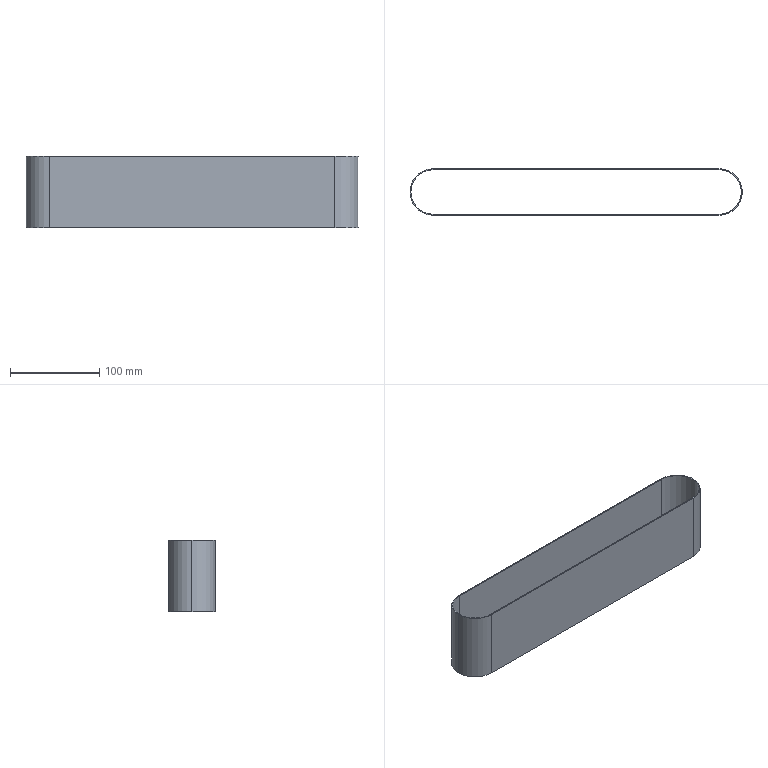Part | SolidWorks | features Extrusion 1 | 1 solid | 12 faces | box 372 x 52 x 80 mm | volume 64018 mm3 | cylinder 6 | plane 6 | commonest cylinder face diameters 50 x3 52 x3
STEP:
#1=CARTESIAN_POINT('',(0.,25.,80.));
#2=VERTEX_POINT('',#1);
#3=CARTESIAN_POINT('',(-25.,0.,80.));
#4=VERTEX_POINT('',#3);
#5=CARTESIAN_POINT('',(0.,0.,80.));
#6=DIRECTION('',(0.,0.,1.));
#7=DIRECTION('',(1.,0.,0.));
#8=AXIS2_PLACEMENT_3D('',#5,#6,#7);
#9=CIRCLE('',#8,25.);
#10=EDGE_CURVE('',#2,#4,#9,.T.);
#11=ORIENTED_EDGE('',*,*,#10,.T.);
#12=CARTESIAN_POINT('',(-25.,0.,0.));
#13=VERTEX_POINT('',#12);
#14=CARTESIAN_POINT('',(-25.,0.,80.));
#15=DIRECTION('',(0.,0.,-1.));
#16=VECTOR('',#15,1000.);
#17=LINE('',#14,#16);
#18=EDGE_CURVE('',#4,#13,#17,.T.);
#19=ORIENTED_EDGE('',*,*,#18,.T.);
#20=CARTESIAN_POINT('',(0.,25.,0.));
#21=VERTEX_POINT('',#20);
#22=CARTESIAN_POINT('',(0.,0.,0.));
#23=DIRECTION('',(0.,0.,1.));
#24=DIRECTION('',(1.,0.,0.));
#25=AXIS2_PLACEMENT_3D('',#22,#23,#24);
#26=CIRCLE('',#25,25.);
#27=EDGE_CURVE('',#21,#13,#26,.T.);
#28=ORIENTED_EDGE('',*,*,#27,.F.);
#29=CARTESIAN_POINT('',(0.,25.,80.));
#30=DIRECTION('',(0.,0.,-1.));
#31=VECTOR('',#30,1000.);
#32=LINE('',#29,#31);
#33=EDGE_CURVE('',#2,#21,#32,.T.);
#34=ORIENTED_EDGE('',*,*,#33,.F.);
#35=EDGE_LOOP('',(#11,#19,#28,#34));
#36=FACE_OUTER_BOUND('',#35,.T.);
#37=CARTESIAN_POINT('',(0.,0.,80.));
#38=DIRECTION('',(0.,0.,-1.));
#39=DIRECTION('',(-1.,0.,0.));
#40=AXIS2_PLACEMENT_3D('',#37,#38,#39);
#41=CYLINDRICAL_SURFACE('',#40,25.);
#42=ADVANCED_FACE('',(#36),#41,.F.);
#43=CARTESIAN_POINT('',(-26.,0.,80.));
#44=VERTEX_POINT('',#43);
#45=CARTESIAN_POINT('',(0.,-26.,80.));
#46=VERTEX_POINT('',#45);
#47=CARTESIAN_POINT('',(0.,0.,80.));
#48=DIRECTION('',(0.,0.,1.));
#49=DIRECTION('',(1.,0.,0.));
#50=AXIS2_PLACEMENT_3D('',#47,#48,#49);
#51=CIRCLE('',#50,26.);
#52=EDGE_CURVE('',#44,#46,#51,.T.);
#53=ORIENTED_EDGE('',*,*,#52,.F.);
#54=CARTESIAN_POINT('',(-26.,0.,0.));
#55=VERTEX_POINT('',#54);
#56=CARTESIAN_POINT('',(-26.,0.,80.));
#57=DIRECTION('',(0.,0.,-1.));
#58=VECTOR('',#57,1000.);
#59=LINE('',#56,#58);
#60=EDGE_CURVE('',#44,#55,#59,.T.);
#61=ORIENTED_EDGE('',*,*,#60,.T.);
#62=CARTESIAN_POINT('',(0.,-26.,0.));
#63=VERTEX_POINT('',#62);
#64=CARTESIAN_POINT('',(0.,0.,0.));
#65=DIRECTION('',(0.,0.,1.));
#66=DIRECTION('',(1.,0.,0.));
#67=AXIS2_PLACEMENT_3D('',#64,#65,#66);
#68=CIRCLE('',#67,26.);
#69=EDGE_CURVE('',#55,#63,#68,.T.);
#70=ORIENTED_EDGE('',*,*,#69,.T.);
#71=CARTESIAN_POINT('',(0.,-26.,80.));
#72=DIRECTION('',(0.,0.,-1.));
#73=VECTOR('',#72,1000.);
#74=LINE('',#71,#73);
#75=EDGE_CURVE('',#46,#63,#74,.T.);
#76=ORIENTED_EDGE('',*,*,#75,.F.);
#77=EDGE_LOOP('',(#53,#61,#70,#76));
#78=FACE_OUTER_BOUND('',#77,.T.);
#79=CARTESIAN_POINT('',(0.,0.,80.));
#80=DIRECTION('',(0.,0.,-1.));
#81=DIRECTION('',(-1.,0.,0.));
#82=AXIS2_PLACEMENT_3D('',#79,#80,#81);
#83=CYLINDRICAL_SURFACE('',#82,26.);
#84=ADVANCED_FACE('',(#78),#83,.T.);
#85=CARTESIAN_POINT('',(0.,26.,80.));
#86=VERTEX_POINT('',#85);
#87=CARTESIAN_POINT('',(0.,0.,80.));
#88=DIRECTION('',(0.,0.,1.));
#89=DIRECTION('',(1.,0.,0.));
#90=AXIS2_PLACEMENT_3D('',#87,#88,#89);
#91=CIRCLE('',#90,26.);
#92=EDGE_CURVE('',#86,#44,#91,.T.);
#93=ORIENTED_EDGE('',*,*,#92,.T.);
#94=ORIENTED_EDGE('',*,*,#52,.T.);
#95=CARTESIAN_POINT('',(320.,-26.,80.));
#96=VERTEX_POINT('',#95);
#97=CARTESIAN_POINT('',(320.,-26.,80.));
#98=DIRECTION('',(1.,0.,0.));
#99=VECTOR('',#98,1000.);
#100=LINE('',#97,#99);
#101=EDGE_CURVE('',#46,#96,#100,.T.);
#102=ORIENTED_EDGE('',*,*,#101,.T.);
#103=CARTESIAN_POINT('',(320.,26.,80.));
#104=VERTEX_POINT('',#103);
#105=CARTESIAN_POINT('',(320.,0.,80.));
#106=DIRECTION('',(0.,0.,1.));
#107=DIRECTION('',(1.,0.,0.));
#108=AXIS2_PLACEMENT_3D('',#105,#106,#107);
#109=CIRCLE('',#108,26.);
#110=EDGE_CURVE('',#96,#104,#109,.T.);
#111=ORIENTED_EDGE('',*,*,#110,.T.);
#112=CARTESIAN_POINT('',(0.,26.,80.));
#113=DIRECTION('',(-1.,0.,0.));
#114=VECTOR('',#113,1000.);
#115=LINE('',#112,#114);
#116=EDGE_CURVE('',#104,#86,#115,.T.);
#117=ORIENTED_EDGE('',*,*,#116,.T.);
#118=EDGE_LOOP('',(#93,#94,#102,#111,#117));
#119=FACE_OUTER_BOUND('',#118,.T.);
#120=CARTESIAN_POINT('',(0.,-25.,80.));
#121=VERTEX_POINT('',#120);
#122=CARTESIAN_POINT('',(320.,-25.,80.));
#123=VERTEX_POINT('',#122);
#124=CARTESIAN_POINT('',(320.,-25.,80.));
#125=DIRECTION('',(1.,0.,0.));
#126=VECTOR('',#125,1000.);
#127=LINE('',#124,#126);
#128=EDGE_CURVE('',#121,#123,#127,.T.);
#129=ORIENTED_EDGE('',*,*,#128,.F.);
#130=CARTESIAN_POINT('',(0.,0.,80.));
#131=DIRECTION('',(0.,0.,1.));
#132=DIRECTION('',(1.,0.,0.));
#133=AXIS2_PLACEMENT_3D('',#130,#131,#132);
#134=CIRCLE('',#133,25.);
#135=EDGE_CURVE('',#4,#121,#134,.T.);
#136=ORIENTED_EDGE('',*,*,#135,.F.);
#137=ORIENTED_EDGE('',*,*,#10,.F.);
#138=CARTESIAN_POINT('',(320.,25.,80.));
#139=VERTEX_POINT('',#138);
#140=CARTESIAN_POINT('',(0.,25.,80.));
#141=DIRECTION('',(-1.,0.,0.));
#142=VECTOR('',#141,1000.);
#143=LINE('',#140,#142);
#144=EDGE_CURVE('',#139,#2,#143,.T.);
#145=ORIENTED_EDGE('',*,*,#144,.F.);
#146=CARTESIAN_POINT('',(320.,0.,80.));
#147=DIRECTION('',(0.,0.,1.));
#148=DIRECTION('',(1.,0.,0.));
#149=AXIS2_PLACEMENT_3D('',#146,#147,#148);
#150=CIRCLE('',#149,25.);
#151=EDGE_CURVE('',#123,#139,#150,.T.);
#152=ORIENTED_EDGE('',*,*,#151,.F.);
#153=EDGE_LOOP('',(#129,#136,#137,#145,#152));
#154=FACE_BOUND('',#153,.T.);
#155=CARTESIAN_POINT('',(0.,0.,80.));
#156=DIRECTION('',(0.,0.,1.));
#157=DIRECTION('',(1.,0.,0.));
#158=AXIS2_PLACEMENT_3D('',#155,#156,#157);
#159=PLANE('',#158);
#160=ADVANCED_FACE('',(#119,#154),#159,.T.);
#161=CARTESIAN_POINT('',(0.,26.,0.));
#162=VERTEX_POINT('',#161);
#163=CARTESIAN_POINT('',(0.,0.,0.));
#164=DIRECTION('',(0.,0.,1.));
#165=DIRECTION('',(1.,0.,0.));
#166=AXIS2_PLACEMENT_3D('',#163,#164,#165);
#167=CIRCLE('',#166,26.);
#168=EDGE_CURVE('',#162,#55,#167,.T.);
#169=ORIENTED_EDGE('',*,*,#168,.F.);
#170=CARTESIAN_POINT('',(320.,26.,0.));
#171=VERTEX_POINT('',#170);
#172=CARTESIAN_POINT('',(0.,26.,0.));
#173=DIRECTION('',(-1.,0.,0.));
#174=VECTOR('',#173,1000.);
#175=LINE('',#172,#174);
#176=EDGE_CURVE('',#171,#162,#175,.T.);
#177=ORIENTED_EDGE('',*,*,#176,.F.);
#178=CARTESIAN_POINT('',(320.,-26.,0.));
#179=VERTEX_POINT('',#178);
#180=CARTESIAN_POINT('',(320.,0.,0.));
#181=DIRECTION('',(0.,0.,1.));
#182=DIRECTION('',(1.,0.,0.));
#183=AXIS2_PLACEMENT_3D('',#180,#181,#182);
#184=CIRCLE('',#183,26.);
#185=EDGE_CURVE('',#179,#171,#184,.T.);
#186=ORIENTED_EDGE('',*,*,#185,.F.);
#187=CARTESIAN_POINT('',(320.,-26.,0.));
#188=DIRECTION('',(1.,0.,0.));
#189=VECTOR('',#188,1000.);
#190=LINE('',#187,#189);
#191=EDGE_CURVE('',#63,#179,#190,.T.);
#192=ORIENTED_EDGE('',*,*,#191,.F.);
#193=ORIENTED_EDGE('',*,*,#69,.F.);
#194=EDGE_LOOP('',(#169,#177,#186,#192,#193));
#195=FACE_OUTER_BOUND('',#194,.T.);
#196=ORIENTED_EDGE('',*,*,#27,.T.);
#197=CARTESIAN_POINT('',(0.,-25.,0.));
#198=VERTEX_POINT('',#197);
#199=CARTESIAN_POINT('',(0.,0.,0.));
#200=DIRECTION('',(0.,0.,1.));
#201=DIRECTION('',(1.,0.,0.));
#202=AXIS2_PLACEMENT_3D('',#199,#200,#201);
#203=CIRCLE('',#202,25.);
#204=EDGE_CURVE('',#13,#198,#203,.T.);
#205=ORIENTED_EDGE('',*,*,#204,.T.);
#206=CARTESIAN_POINT('',(320.,-25.,0.));
#207=VERTEX_POINT('',#206);
#208=CARTESIAN_POINT('',(320.,-25.,0.));
#209=DIRECTION('',(1.,0.,0.));
#210=VECTOR('',#209,1000.);
#211=LINE('',#208,#210);
#212=EDGE_CURVE('',#198,#207,#211,.T.);
#213=ORIENTED_EDGE('',*,*,#212,.T.);
#214=CARTESIAN_POINT('',(320.,25.,0.));
#215=VERTEX_POINT('',#214);
#216=CARTESIAN_POINT('',(320.,0.,0.));
#217=DIRECTION('',(0.,0.,1.));
#218=DIRECTION('',(1.,0.,0.));
#219=AXIS2_PLACEMENT_3D('',#216,#217,#218);
#220=CIRCLE('',#219,25.);
#221=EDGE_CURVE('',#207,#215,#220,.T.);
#222=ORIENTED_EDGE('',*,*,#221,.T.);
#223=CARTESIAN_POINT('',(0.,25.,0.));
#224=DIRECTION('',(-1.,0.,0.));
#225=VECTOR('',#224,1000.);
#226=LINE('',#223,#225);
#227=EDGE_CURVE('',#215,#21,#226,.T.);
#228=ORIENTED_EDGE('',*,*,#227,.T.);
#229=EDGE_LOOP('',(#196,#205,#213,#222,#228));
#230=FACE_BOUND('',#229,.T.);
#231=CARTESIAN_POINT('',(0.,0.,0.));
#232=DIRECTION('',(0.,0.,1.));
#233=DIRECTION('',(1.,0.,0.));
#234=AXIS2_PLACEMENT_3D('',#231,#232,#233);
#235=PLANE('',#234);
#236=ADVANCED_FACE('',(#195,#230),#235,.F.);
#237=ORIENTED_EDGE('',*,*,#60,.F.);
#238=ORIENTED_EDGE('',*,*,#92,.F.);
#239=CARTESIAN_POINT('',(0.,26.,80.));
#240=DIRECTION('',(0.,0.,-1.));
#241=VECTOR('',#240,1000.);
#242=LINE('',#239,#241);
#243=EDGE_CURVE('',#86,#162,#242,.T.);
#244=ORIENTED_EDGE('',*,*,#243,.T.);
#245=ORIENTED_EDGE('',*,*,#168,.T.);
#246=EDGE_LOOP('',(#237,#238,#244,#245));
#247=FACE_OUTER_BOUND('',#246,.T.);
#248=CARTESIAN_POINT('',(0.,0.,80.));
#249=DIRECTION('',(0.,0.,-1.));
#250=DIRECTION('',(-1.,0.,0.));
#251=AXIS2_PLACEMENT_3D('',#248,#249,#250);
#252=CYLINDRICAL_SURFACE('',#251,26.);
#253=ADVANCED_FACE('',(#247),#252,.T.);
#254=ORIENTED_EDGE('',*,*,#191,.T.);
#255=CARTESIAN_POINT('',(320.,-26.,80.));
#256=DIRECTION('',(0.,0.,-1.));
#257=VECTOR('',#256,1000.);
#258=LINE('',#255,#257);
#259=EDGE_CURVE('',#96,#179,#258,.T.);
#260=ORIENTED_EDGE('',*,*,#259,.F.);
#261=ORIENTED_EDGE('',*,*,#101,.F.);
#262=ORIENTED_EDGE('',*,*,#75,.T.);
#263=EDGE_LOOP('',(#254,#260,#261,#262));
#264=FACE_OUTER_BOUND('',#263,.T.);
#265=CARTESIAN_POINT('',(320.,-26.,80.));
#266=DIRECTION('',(0.,1.,0.));
#267=DIRECTION('',(-1.,0.,0.));
#268=AXIS2_PLACEMENT_3D('',#265,#266,#267);
#269=PLANE('',#268);
#270=ADVANCED_FACE('',(#264),#269,.F.);
#271=ORIENTED_EDGE('',*,*,#185,.T.);
#272=CARTESIAN_POINT('',(320.,26.,80.));
#273=DIRECTION('',(0.,0.,-1.));
#274=VECTOR('',#273,1000.);
#275=LINE('',#272,#274);
#276=EDGE_CURVE('',#104,#171,#275,.T.);
#277=ORIENTED_EDGE('',*,*,#276,.F.);
#278=ORIENTED_EDGE('',*,*,#110,.F.);
#279=ORIENTED_EDGE('',*,*,#259,.T.);
#280=EDGE_LOOP('',(#271,#277,#278,#279));
#281=FACE_OUTER_BOUND('',#280,.T.);
#282=CARTESIAN_POINT('',(320.,0.,80.));
#283=DIRECTION('',(0.,0.,-1.));
#284=DIRECTION('',(-1.,0.,0.));
#285=AXIS2_PLACEMENT_3D('',#282,#283,#284);
#286=CYLINDRICAL_SURFACE('',#285,26.);
#287=ADVANCED_FACE('',(#281),#286,.T.);
#288=ORIENTED_EDGE('',*,*,#176,.T.);
#289=ORIENTED_EDGE('',*,*,#243,.F.);
#290=ORIENTED_EDGE('',*,*,#116,.F.);
#291=ORIENTED_EDGE('',*,*,#276,.T.);
#292=EDGE_LOOP('',(#288,#289,#290,#291));
#293=FACE_OUTER_BOUND('',#292,.T.);
#294=CARTESIAN_POINT('',(0.,26.,80.));
#295=DIRECTION('',(0.,-1.,0.));
#296=DIRECTION('',(1.,0.,0.));
#297=AXIS2_PLACEMENT_3D('',#294,#295,#296);
#298=PLANE('',#297);
#299=ADVANCED_FACE('',(#293),#298,.F.);
#300=ORIENTED_EDGE('',*,*,#18,.F.);
#301=ORIENTED_EDGE('',*,*,#135,.T.);
#302=CARTESIAN_POINT('',(0.,-25.,80.));
#303=DIRECTION('',(0.,0.,-1.));
#304=VECTOR('',#303,1000.);
#305=LINE('',#302,#304);
#306=EDGE_CURVE('',#121,#198,#305,.T.);
#307=ORIENTED_EDGE('',*,*,#306,.T.);
#308=ORIENTED_EDGE('',*,*,#204,.F.);
#309=EDGE_LOOP('',(#300,#301,#307,#308));
#310=FACE_OUTER_BOUND('',#309,.T.);
#311=CARTESIAN_POINT('',(0.,0.,80.));
#312=DIRECTION('',(0.,0.,-1.));
#313=DIRECTION('',(-1.,0.,0.));
#314=AXIS2_PLACEMENT_3D('',#311,#312,#313);
#315=CYLINDRICAL_SURFACE('',#314,25.);
#316=ADVANCED_FACE('',(#310),#315,.F.);
#317=ORIENTED_EDGE('',*,*,#212,.F.);
#318=ORIENTED_EDGE('',*,*,#306,.F.);
#319=ORIENTED_EDGE('',*,*,#128,.T.);
#320=CARTESIAN_POINT('',(320.,-25.,80.));
#321=DIRECTION('',(0.,0.,-1.));
#322=VECTOR('',#321,1000.);
#323=LINE('',#320,#322);
#324=EDGE_CURVE('',#123,#207,#323,.T.);
#325=ORIENTED_EDGE('',*,*,#324,.T.);
#326=EDGE_LOOP('',(#317,#318,#319,#325));
#327=FACE_OUTER_BOUND('',#326,.T.);
#328=CARTESIAN_POINT('',(320.,-25.,80.));
#329=DIRECTION('',(0.,1.,0.));
#330=DIRECTION('',(-1.,0.,0.));
#331=AXIS2_PLACEMENT_3D('',#328,#329,#330);
#332=PLANE('',#331);
#333=ADVANCED_FACE('',(#327),#332,.T.);
#334=ORIENTED_EDGE('',*,*,#221,.F.);
#335=ORIENTED_EDGE('',*,*,#324,.F.);
#336=ORIENTED_EDGE('',*,*,#151,.T.);
#337=CARTESIAN_POINT('',(320.,25.,80.));
#338=DIRECTION('',(0.,0.,-1.));
#339=VECTOR('',#338,1000.);
#340=LINE('',#337,#339);
#341=EDGE_CURVE('',#139,#215,#340,.T.);
#342=ORIENTED_EDGE('',*,*,#341,.T.);
#343=EDGE_LOOP('',(#334,#335,#336,#342));
#344=FACE_OUTER_BOUND('',#343,.T.);
#345=CARTESIAN_POINT('',(320.,0.,80.));
#346=DIRECTION('',(0.,0.,-1.));
#347=DIRECTION('',(-1.,0.,0.));
#348=AXIS2_PLACEMENT_3D('',#345,#346,#347);
#349=CYLINDRICAL_SURFACE('',#348,25.);
#350=ADVANCED_FACE('',(#344),#349,.F.);
#351=ORIENTED_EDGE('',*,*,#227,.F.);
#352=ORIENTED_EDGE('',*,*,#341,.F.);
#353=ORIENTED_EDGE('',*,*,#144,.T.);
#354=ORIENTED_EDGE('',*,*,#33,.T.);
#355=EDGE_LOOP('',(#351,#352,#353,#354));
#356=FACE_OUTER_BOUND('',#355,.T.);
#357=CARTESIAN_POINT('',(0.,25.,80.));
#358=DIRECTION('',(0.,-1.,0.));
#359=DIRECTION('',(1.,0.,0.));
#360=AXIS2_PLACEMENT_3D('',#357,#358,#359);
#361=PLANE('',#360);
#362=ADVANCED_FACE('',(#356),#361,.T.);
#363=CLOSED_SHELL('',(#42,#84,#160,#236,#253,#270,#287,#299,#316,#333,#350,#362));
#364=MANIFOLD_SOLID_BREP('',#363);
#365=CARTESIAN_POINT('',(0.,0.,0.));
#366=DIRECTION('',(0.,0.,1.));
#367=DIRECTION('',(1.,0.,0.));
#368=AXIS2_PLACEMENT_3D('',#365,#366,#367);
#369=(LENGTH_UNIT()NAMED_UNIT(*)SI_UNIT(.MILLI.,.METRE.));
#370=UNCERTAINTY_MEASURE_WITH_UNIT(LENGTH_MEASURE(0.00001),#369,'','');
#371=(NAMED_UNIT(*)PLANE_ANGLE_UNIT()SI_UNIT($,.RADIAN.));
#372=(NAMED_UNIT(*)SI_UNIT($,.STERADIAN.)SOLID_ANGLE_UNIT());
#373=(GEOMETRIC_REPRESENTATION_CONTEXT(3)GLOBAL_UNCERTAINTY_ASSIGNED_CONTEXT((#370))GLOBAL_UNIT_ASSIGNED_CONTEXT((#369,#371,#372))REPRESENTATION_CONTEXT('',''));
#374=ADVANCED_BREP_SHAPE_REPRESENTATION('',(#364,#368),#373);